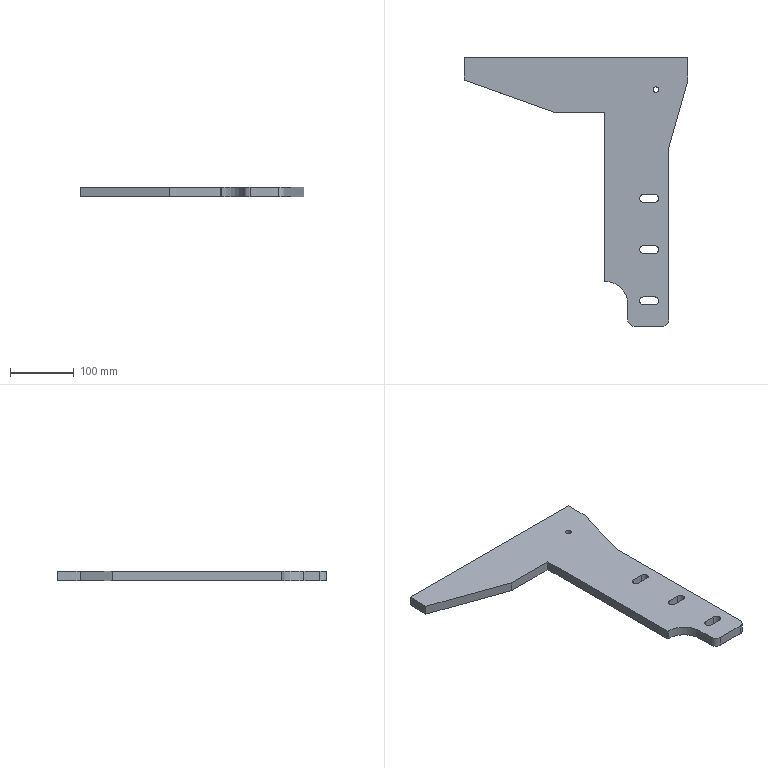Part | STEP file | Input 56 | 1 solid | 33 faces | box 350 x 420 x 15 mm | volume 847153 mm3 | plane 19 | cylinder 14 | commonest cylinder face diameters 12 x9 8.8 x2 20 x2 70 x1